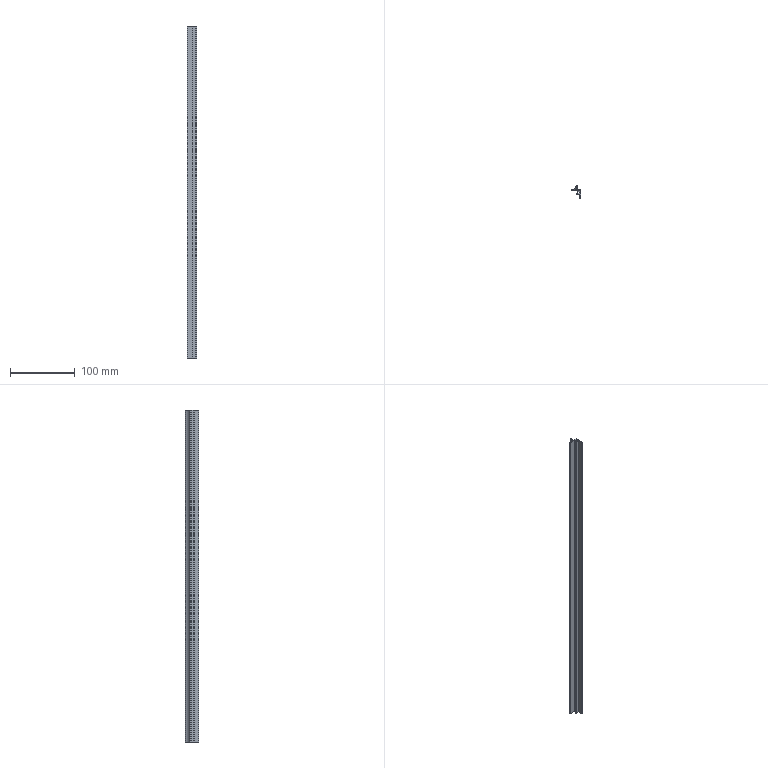Part | SolidWorks | features BaseBody 1, ICE 1, MoveFace 1 | 1 solid | 27 faces | box 14 x 20.3 x 513 mm | volume 26120 mm3 | plane 20 | cylinder 7 | commonest cylinder face diameters 0.387 x2 0.8 x2 0.4 x1 20 x1 22 x1
STEP:
#1=CARTESIAN_POINT('',(-5.304,-0.625,200.));
#2=VERTEX_POINT('',#1);
#3=CARTESIAN_POINT('',(-5.449,-0.8125,200.));
#4=VERTEX_POINT('',#3);
#5=CARTESIAN_POINT('',(-5.255,-0.8125,200.));
#6=DIRECTION('',(0.,0.,1.));
#7=DIRECTION('',(-1.,0.,0.));
#8=AXIS2_PLACEMENT_3D('',#5,#6,#7);
#9=CIRCLE('',#8,0.1937);
#10=EDGE_CURVE('',#2,#4,#9,.T.);
#11=ORIENTED_EDGE('',*,*,#10,.T.);
#12=CARTESIAN_POINT('',(-5.449,-0.8125,-313.));
#13=VERTEX_POINT('',#12);
#14=CARTESIAN_POINT('',(-5.449,-0.8125,230.));
#15=DIRECTION('',(0.,0.,-1.));
#16=VECTOR('',#15,1000.);
#17=LINE('',#14,#16);
#18=EDGE_CURVE('',#4,#13,#17,.T.);
#19=ORIENTED_EDGE('',*,*,#18,.T.);
#20=CARTESIAN_POINT('',(-5.304,-0.625,-313.));
#21=VERTEX_POINT('',#20);
#22=CARTESIAN_POINT('',(-5.255,-0.8125,-313.));
#23=DIRECTION('',(0.,0.,-1.));
#24=DIRECTION('',(1.,0.,0.));
#25=AXIS2_PLACEMENT_3D('',#22,#23,#24);
#26=CIRCLE('',#25,0.1937);
#27=EDGE_CURVE('',#13,#21,#26,.T.);
#28=ORIENTED_EDGE('',*,*,#27,.T.);
#29=CARTESIAN_POINT('',(-5.304,-0.625,230.));
#30=DIRECTION('',(0.,0.,-1.));
#31=VECTOR('',#30,1000.);
#32=LINE('',#29,#31);
#33=EDGE_CURVE('',#2,#21,#32,.T.);
#34=ORIENTED_EDGE('',*,*,#33,.F.);
#35=EDGE_LOOP('',(#11,#19,#28,#34));
#36=FACE_OUTER_BOUND('',#35,.T.);
#37=CARTESIAN_POINT('',(-5.255,-0.8125,230.));
#38=DIRECTION('',(0.,0.,-1.));
#39=DIRECTION('',(-1.,0.,0.));
#40=AXIS2_PLACEMENT_3D('',#37,#38,#39);
#41=CYLINDRICAL_SURFACE('',#40,0.1937);
#42=ADVANCED_FACE('',(#36),#41,.F.);
#43=CARTESIAN_POINT('',(5.,-1.,-313.));
#44=VERTEX_POINT('',#43);
#45=CARTESIAN_POINT('',(5.,-14.3,-313.));
#46=VERTEX_POINT('',#45);
#47=CARTESIAN_POINT('',(5.,29.623,-313.));
#48=DIRECTION('',(0.,-1.,0.));
#49=VECTOR('',#48,1000.);
#50=LINE('',#47,#49);
#51=EDGE_CURVE('',#44,#46,#50,.T.);
#52=ORIENTED_EDGE('',*,*,#51,.F.);
#53=CARTESIAN_POINT('',(5.,-1.,200.));
#54=VERTEX_POINT('',#53);
#55=CARTESIAN_POINT('',(5.,-1.,230.));
#56=DIRECTION('',(0.,0.,-1.));
#57=VECTOR('',#56,1000.);
#58=LINE('',#55,#57);
#59=EDGE_CURVE('',#54,#44,#58,.T.);
#60=ORIENTED_EDGE('',*,*,#59,.F.);
#61=CARTESIAN_POINT('',(5.,-14.3,200.));
#62=VERTEX_POINT('',#61);
#63=CARTESIAN_POINT('',(5.,-14.3,200.));
#64=DIRECTION('',(0.,1.,0.));
#65=VECTOR('',#64,1000.);
#66=LINE('',#63,#65);
#67=EDGE_CURVE('',#62,#54,#66,.T.);
#68=ORIENTED_EDGE('',*,*,#67,.F.);
#69=CARTESIAN_POINT('',(5.,-14.3,230.));
#70=DIRECTION('',(0.,0.,1.));
#71=VECTOR('',#70,1000.);
#72=LINE('',#69,#71);
#73=EDGE_CURVE('',#46,#62,#72,.T.);
#74=ORIENTED_EDGE('',*,*,#73,.F.);
#75=EDGE_LOOP('',(#52,#60,#68,#74));
#76=FACE_OUTER_BOUND('',#75,.T.);
#77=CARTESIAN_POINT('',(5.,-14.3,230.));
#78=DIRECTION('',(-1.,0.,0.));
#79=DIRECTION('',(0.,0.,1.));
#80=AXIS2_PLACEMENT_3D('',#77,#78,#79);
#81=PLANE('',#80);
#82=ADVANCED_FACE('',(#76),#81,.F.);
#83=CARTESIAN_POINT('',(-9.,-2.,-313.));
#84=VERTEX_POINT('',#83);
#85=CARTESIAN_POINT('',(-9.,-2.,200.));
#86=VERTEX_POINT('',#85);
#87=CARTESIAN_POINT('',(-9.,-2.,230.));
#88=DIRECTION('',(0.,0.,1.));
#89=VECTOR('',#88,1000.);
#90=LINE('',#87,#89);
#91=EDGE_CURVE('',#84,#86,#90,.T.);
#92=ORIENTED_EDGE('',*,*,#91,.F.);
#93=CARTESIAN_POINT('',(0.9,-2.,-313.));
#94=VERTEX_POINT('',#93);
#95=CARTESIAN_POINT('',(5.,-2.,-313.));
#96=DIRECTION('',(-1.,0.,0.));
#97=VECTOR('',#96,1000.);
#98=LINE('',#95,#97);
#99=EDGE_CURVE('',#94,#84,#98,.T.);
#100=ORIENTED_EDGE('',*,*,#99,.F.);
#101=CARTESIAN_POINT('',(0.9,-2.,200.));
#102=VERTEX_POINT('',#101);
#103=CARTESIAN_POINT('',(0.9,-2.,230.));
#104=DIRECTION('',(0.,0.,-1.));
#105=VECTOR('',#104,1000.);
#106=LINE('',#103,#105);
#107=EDGE_CURVE('',#102,#94,#106,.T.);
#108=ORIENTED_EDGE('',*,*,#107,.F.);
#109=CARTESIAN_POINT('',(5.,-2.,200.));
#110=DIRECTION('',(1.,0.,0.));
#111=VECTOR('',#110,1000.);
#112=LINE('',#109,#111);
#113=EDGE_CURVE('',#86,#102,#112,.T.);
#114=ORIENTED_EDGE('',*,*,#113,.F.);
#115=EDGE_LOOP('',(#92,#100,#108,#114));
#116=FACE_OUTER_BOUND('',#115,.T.);
#117=CARTESIAN_POINT('',(-9.,-2.,230.));
#118=DIRECTION('',(0.,1.,0.));
#119=DIRECTION('',(0.,0.,1.));
#120=AXIS2_PLACEMENT_3D('',#117,#118,#119);
#121=PLANE('',#120);
#122=ADVANCED_FACE('',(#116),#121,.F.);
#123=CARTESIAN_POINT('',(4.,-6.,200.));
#124=VERTEX_POINT('',#123);
#125=CARTESIAN_POINT('',(4.,-3.,200.));
#126=VERTEX_POINT('',#125);
#127=CARTESIAN_POINT('',(4.,29.623,200.));
#128=DIRECTION('',(0.,1.,0.));
#129=VECTOR('',#128,1000.);
#130=LINE('',#127,#129);
#131=EDGE_CURVE('',#124,#126,#130,.T.);
#132=ORIENTED_EDGE('',*,*,#131,.F.);
#133=CARTESIAN_POINT('',(1.,-6.,200.));
#134=VERTEX_POINT('',#133);
#135=CARTESIAN_POINT('',(5.,-6.,200.));
#136=DIRECTION('',(1.,0.,0.));
#137=VECTOR('',#136,1000.);
#138=LINE('',#135,#137);
#139=EDGE_CURVE('',#134,#124,#138,.T.);
#140=ORIENTED_EDGE('',*,*,#139,.F.);
#141=CARTESIAN_POINT('',(1.,-6.7,200.));
#142=VERTEX_POINT('',#141);
#143=CARTESIAN_POINT('',(1.,-6.,200.));
#144=DIRECTION('',(0.,-1.,0.));
#145=VECTOR('',#144,1000.);
#146=LINE('',#143,#145);
#147=EDGE_CURVE('',#134,#142,#146,.T.);
#148=ORIENTED_EDGE('',*,*,#147,.T.);
#149=CARTESIAN_POINT('',(-1.7,-6.7,200.));
#150=VERTEX_POINT('',#149);
#151=CARTESIAN_POINT('',(5.,-6.7,200.));
#152=DIRECTION('',(1.,0.,0.));
#153=VECTOR('',#152,1000.);
#154=LINE('',#151,#153);
#155=EDGE_CURVE('',#150,#142,#154,.T.);
#156=ORIENTED_EDGE('',*,*,#155,.F.);
#157=CARTESIAN_POINT('',(-1.7,-7.7,200.));
#158=VERTEX_POINT('',#157);
#159=CARTESIAN_POINT('',(-1.7,-6.7,200.));
#160=DIRECTION('',(0.,-1.,0.));
#161=VECTOR('',#160,1000.);
#162=LINE('',#159,#161);
#163=EDGE_CURVE('',#150,#158,#162,.T.);
#164=ORIENTED_EDGE('',*,*,#163,.T.);
#165=CARTESIAN_POINT('',(4.,-7.7,200.));
#166=VERTEX_POINT('',#165);
#167=CARTESIAN_POINT('',(5.,-7.7,200.));
#168=DIRECTION('',(-1.,0.,0.));
#169=VECTOR('',#168,1000.);
#170=LINE('',#167,#169);
#171=EDGE_CURVE('',#166,#158,#170,.T.);
#172=ORIENTED_EDGE('',*,*,#171,.F.);
#173=CARTESIAN_POINT('',(4.,-14.3,200.));
#174=VERTEX_POINT('',#173);
#175=CARTESIAN_POINT('',(4.,29.623,200.));
#176=DIRECTION('',(0.,1.,0.));
#177=VECTOR('',#176,1000.);
#178=LINE('',#175,#177);
#179=EDGE_CURVE('',#174,#166,#178,.T.);
#180=ORIENTED_EDGE('',*,*,#179,.F.);
#181=CARTESIAN_POINT('',(5.,-14.3,200.));
#182=DIRECTION('',(-1.,0.,0.));
#183=VECTOR('',#182,1000.);
#184=LINE('',#181,#183);
#185=EDGE_CURVE('',#62,#174,#184,.T.);
#186=ORIENTED_EDGE('',*,*,#185,.F.);
#187=ORIENTED_EDGE('',*,*,#67,.T.);
#188=CARTESIAN_POINT('',(-5.207,-1.,200.));
#189=VERTEX_POINT('',#188);
#190=CARTESIAN_POINT('',(5.,-1.,200.));
#191=DIRECTION('',(1.,0.,0.));
#192=VECTOR('',#191,1000.);
#193=LINE('',#190,#192);
#194=EDGE_CURVE('',#189,#54,#193,.T.);
#195=ORIENTED_EDGE('',*,*,#194,.F.);
#196=CARTESIAN_POINT('',(-5.255,-0.8125,200.));
#197=DIRECTION('',(0.,0.,1.));
#198=DIRECTION('',(-1.,0.,0.));
#199=AXIS2_PLACEMENT_3D('',#196,#197,#198);
#200=CIRCLE('',#199,0.1937);
#201=EDGE_CURVE('',#4,#189,#200,.T.);
#202=ORIENTED_EDGE('',*,*,#201,.F.);
#203=ORIENTED_EDGE('',*,*,#10,.F.);
#204=CARTESIAN_POINT('',(-1.368,3.063,200.));
#205=VERTEX_POINT('',#204);
#206=CARTESIAN_POINT('',(-10.628,9.,200.));
#207=DIRECTION('',(0.,0.,1.));
#208=DIRECTION('',(-1.,0.,0.));
#209=AXIS2_PLACEMENT_3D('',#206,#207,#208);
#210=CIRCLE('',#209,11.);
#211=EDGE_CURVE('',#2,#205,#210,.T.);
#212=ORIENTED_EDGE('',*,*,#211,.T.);
#213=CARTESIAN_POINT('',(-1.,2.955,200.));
#214=VERTEX_POINT('',#213);
#215=CARTESIAN_POINT('',(-1.2,2.955,200.));
#216=DIRECTION('',(0.,0.,1.));
#217=DIRECTION('',(-1.,0.,0.));
#218=AXIS2_PLACEMENT_3D('',#215,#216,#217);
#219=CIRCLE('',#218,0.2);
#220=EDGE_CURVE('',#214,#205,#219,.T.);
#221=ORIENTED_EDGE('',*,*,#220,.F.);
#222=CARTESIAN_POINT('',(-1.,1.5,200.));
#223=VERTEX_POINT('',#222);
#224=CARTESIAN_POINT('',(-1.,2.955,200.));
#225=DIRECTION('',(0.,1.,0.));
#226=VECTOR('',#225,1000.);
#227=LINE('',#224,#226);
#228=EDGE_CURVE('',#223,#214,#227,.T.);
#229=ORIENTED_EDGE('',*,*,#228,.F.);
#230=CARTESIAN_POINT('',(0.,1.5,200.));
#231=VERTEX_POINT('',#230);
#232=CARTESIAN_POINT('',(-1.,1.5,200.));
#233=DIRECTION('',(-1.,0.,0.));
#234=VECTOR('',#233,1000.);
#235=LINE('',#232,#234);
#236=EDGE_CURVE('',#231,#223,#235,.T.);
#237=ORIENTED_EDGE('',*,*,#236,.F.);
#238=CARTESIAN_POINT('',(0.,6.,200.));
#239=VERTEX_POINT('',#238);
#240=CARTESIAN_POINT('',(0.,1.5,200.));
#241=DIRECTION('',(0.,-1.,0.));
#242=VECTOR('',#241,1000.);
#243=LINE('',#240,#242);
#244=EDGE_CURVE('',#239,#231,#243,.T.);
#245=ORIENTED_EDGE('',*,*,#244,.F.);
#246=CARTESIAN_POINT('',(-0.8,6.,200.));
#247=VERTEX_POINT('',#246);
#248=CARTESIAN_POINT('',(0.,6.,200.));
#249=DIRECTION('',(1.,0.,0.));
#250=VECTOR('',#249,1000.);
#251=LINE('',#248,#250);
#252=EDGE_CURVE('',#247,#239,#251,.T.);
#253=ORIENTED_EDGE('',*,*,#252,.F.);
#254=CARTESIAN_POINT('',(-1.178,5.731,200.));
#255=VERTEX_POINT('',#254);
#256=CARTESIAN_POINT('',(-0.8,5.6,200.));
#257=DIRECTION('',(0.,0.,1.));
#258=DIRECTION('',(-1.,0.,0.));
#259=AXIS2_PLACEMENT_3D('',#256,#257,#258);
#260=CIRCLE('',#259,0.4);
#261=EDGE_CURVE('',#247,#255,#260,.T.);
#262=ORIENTED_EDGE('',*,*,#261,.T.);
#263=CARTESIAN_POINT('',(-8.678,-0.8077,200.));
#264=VERTEX_POINT('',#263);
#265=CARTESIAN_POINT('',(-10.628,9.,200.));
#266=DIRECTION('',(0.,0.,1.));
#267=DIRECTION('',(-1.,0.,0.));
#268=AXIS2_PLACEMENT_3D('',#265,#266,#267);
#269=CIRCLE('',#268,10.);
#270=EDGE_CURVE('',#264,#255,#269,.T.);
#271=ORIENTED_EDGE('',*,*,#270,.F.);
#272=CARTESIAN_POINT('',(-9.,-1.2,200.));
#273=VERTEX_POINT('',#272);
#274=CARTESIAN_POINT('',(-8.6,-1.2,200.));
#275=DIRECTION('',(0.,0.,1.));
#276=DIRECTION('',(-1.,0.,0.));
#277=AXIS2_PLACEMENT_3D('',#274,#275,#276);
#278=CIRCLE('',#277,0.4);
#279=EDGE_CURVE('',#264,#273,#278,.T.);
#280=ORIENTED_EDGE('',*,*,#279,.T.);
#281=CARTESIAN_POINT('',(-9.,8.,200.));
#282=DIRECTION('',(0.,-1.,0.));
#283=VECTOR('',#282,1000.);
#284=LINE('',#281,#283);
#285=EDGE_CURVE('',#273,#86,#284,.T.);
#286=ORIENTED_EDGE('',*,*,#285,.T.);
#287=ORIENTED_EDGE('',*,*,#113,.T.);
#288=CARTESIAN_POINT('',(0.9,-3.,200.));
#289=VERTEX_POINT('',#288);
#290=CARTESIAN_POINT('',(0.9,29.623,200.));
#291=DIRECTION('',(0.,1.,0.));
#292=VECTOR('',#291,1000.);
#293=LINE('',#290,#292);
#294=EDGE_CURVE('',#289,#102,#293,.T.);
#295=ORIENTED_EDGE('',*,*,#294,.F.);
#296=CARTESIAN_POINT('',(5.,-3.,200.));
#297=DIRECTION('',(-1.,0.,0.));
#298=VECTOR('',#297,1000.);
#299=LINE('',#296,#298);
#300=EDGE_CURVE('',#126,#289,#299,.T.);
#301=ORIENTED_EDGE('',*,*,#300,.F.);
#302=EDGE_LOOP('',(#132,#140,#148,#156,#164,#172,#180,#186,#187,#195,#202,#203,#212,#221,#229,#237,#245,#253,#262,#271,#280,#286,#287,#295,#301));
#303=FACE_OUTER_BOUND('',#302,.T.);
#304=CARTESIAN_POINT('',(5.,29.623,200.));
#305=DIRECTION('',(0.,0.,-1.));
#306=DIRECTION('',(-1.,0.,0.));
#307=AXIS2_PLACEMENT_3D('',#304,#305,#306);
#308=PLANE('',#307);
#309=ADVANCED_FACE('',(#303),#308,.F.);
#310=ORIENTED_EDGE('',*,*,#185,.T.);
#311=CARTESIAN_POINT('',(4.,-14.3,-313.));
#312=VERTEX_POINT('',#311);
#313=CARTESIAN_POINT('',(4.,-14.3,230.));
#314=DIRECTION('',(0.,0.,1.));
#315=VECTOR('',#314,1000.);
#316=LINE('',#313,#315);
#317=EDGE_CURVE('',#312,#174,#316,.T.);
#318=ORIENTED_EDGE('',*,*,#317,.F.);
#319=CARTESIAN_POINT('',(5.,-14.3,-313.));
#320=DIRECTION('',(-1.,0.,0.));
#321=VECTOR('',#320,1000.);
#322=LINE('',#319,#321);
#323=EDGE_CURVE('',#46,#312,#322,.T.);
#324=ORIENTED_EDGE('',*,*,#323,.F.);
#325=ORIENTED_EDGE('',*,*,#73,.T.);
#326=EDGE_LOOP('',(#310,#318,#324,#325));
#327=FACE_OUTER_BOUND('',#326,.T.);
#328=CARTESIAN_POINT('',(4.,-14.3,230.));
#329=DIRECTION('',(0.,1.,0.));
#330=DIRECTION('',(0.,0.,1.));
#331=AXIS2_PLACEMENT_3D('',#328,#329,#330);
#332=PLANE('',#331);
#333=ADVANCED_FACE('',(#327),#332,.F.);
#334=ORIENTED_EDGE('',*,*,#51,.T.);
#335=ORIENTED_EDGE('',*,*,#323,.T.);
#336=CARTESIAN_POINT('',(4.,-7.7,-313.));
#337=VERTEX_POINT('',#336);
#338=CARTESIAN_POINT('',(4.,-7.7,-313.));
#339=DIRECTION('',(0.,-1.,0.));
#340=VECTOR('',#339,1000.);
#341=LINE('',#338,#340);
#342=EDGE_CURVE('',#337,#312,#341,.T.);
#343=ORIENTED_EDGE('',*,*,#342,.F.);
#344=CARTESIAN_POINT('',(-1.7,-7.7,-313.));
#345=VERTEX_POINT('',#344);
#346=CARTESIAN_POINT('',(-1.7,-7.7,-313.));
#347=DIRECTION('',(1.,0.,0.));
#348=VECTOR('',#347,1000.);
#349=LINE('',#346,#348);
#350=EDGE_CURVE('',#345,#337,#349,.T.);
#351=ORIENTED_EDGE('',*,*,#350,.F.);
#352=CARTESIAN_POINT('',(-1.7,-6.7,-313.));
#353=VERTEX_POINT('',#352);
#354=CARTESIAN_POINT('',(-1.7,29.623,-313.));
#355=DIRECTION('',(0.,1.,0.));
#356=VECTOR('',#355,1000.);
#357=LINE('',#354,#356);
#358=EDGE_CURVE('',#345,#353,#357,.T.);
#359=ORIENTED_EDGE('',*,*,#358,.T.);
#360=CARTESIAN_POINT('',(1.,-6.7,-313.));
#361=VERTEX_POINT('',#360);
#362=CARTESIAN_POINT('',(1.,-6.7,-313.));
#363=DIRECTION('',(-1.,0.,0.));
#364=VECTOR('',#363,1000.);
#365=LINE('',#362,#364);
#366=EDGE_CURVE('',#361,#353,#365,.T.);
#367=ORIENTED_EDGE('',*,*,#366,.F.);
#368=CARTESIAN_POINT('',(1.,-6.,-313.));
#369=VERTEX_POINT('',#368);
#370=CARTESIAN_POINT('',(1.,29.623,-313.));
#371=DIRECTION('',(0.,1.,0.));
#372=VECTOR('',#371,1000.);
#373=LINE('',#370,#372);
#374=EDGE_CURVE('',#361,#369,#373,.T.);
#375=ORIENTED_EDGE('',*,*,#374,.T.);
#376=CARTESIAN_POINT('',(4.,-6.,-313.));
#377=VERTEX_POINT('',#376);
#378=CARTESIAN_POINT('',(4.,-6.,-313.));
#379=DIRECTION('',(-1.,0.,0.));
#380=VECTOR('',#379,1000.);
#381=LINE('',#378,#380);
#382=EDGE_CURVE('',#377,#369,#381,.T.);
#383=ORIENTED_EDGE('',*,*,#382,.F.);
#384=CARTESIAN_POINT('',(4.,-3.,-313.));
#385=VERTEX_POINT('',#384);
#386=CARTESIAN_POINT('',(4.,-3.,-313.));
#387=DIRECTION('',(0.,-1.,0.));
#388=VECTOR('',#387,1000.);
#389=LINE('',#386,#388);
#390=EDGE_CURVE('',#385,#377,#389,.T.);
#391=ORIENTED_EDGE('',*,*,#390,.F.);
#392=CARTESIAN_POINT('',(0.9,-3.,-313.));
#393=VERTEX_POINT('',#392);
#394=CARTESIAN_POINT('',(0.9,-3.,-313.));
#395=DIRECTION('',(1.,0.,0.));
#396=VECTOR('',#395,1000.);
#397=LINE('',#394,#396);
#398=EDGE_CURVE('',#393,#385,#397,.T.);
#399=ORIENTED_EDGE('',*,*,#398,.F.);
#400=CARTESIAN_POINT('',(0.9,-2.,-313.));
#401=DIRECTION('',(0.,-1.,0.));
#402=VECTOR('',#401,1000.);
#403=LINE('',#400,#402);
#404=EDGE_CURVE('',#94,#393,#403,.T.);
#405=ORIENTED_EDGE('',*,*,#404,.F.);
#406=ORIENTED_EDGE('',*,*,#99,.T.);
#407=CARTESIAN_POINT('',(-9.,-1.2,-313.));
#408=VERTEX_POINT('',#407);
#409=CARTESIAN_POINT('',(-9.,-1.2,-313.));
#410=DIRECTION('',(0.,-1.,0.));
#411=VECTOR('',#410,1000.);
#412=LINE('',#409,#411);
#413=EDGE_CURVE('',#408,#84,#412,.T.);
#414=ORIENTED_EDGE('',*,*,#413,.F.);
#415=CARTESIAN_POINT('',(-8.678,-0.8077,-313.));
#416=VERTEX_POINT('',#415);
#417=CARTESIAN_POINT('',(-8.6,-1.2,-313.));
#418=DIRECTION('',(0.,0.,-1.));
#419=DIRECTION('',(1.,0.,0.));
#420=AXIS2_PLACEMENT_3D('',#417,#418,#419);
#421=CIRCLE('',#420,0.4);
#422=EDGE_CURVE('',#408,#416,#421,.T.);
#423=ORIENTED_EDGE('',*,*,#422,.T.);
#424=CARTESIAN_POINT('',(-1.178,5.731,-313.));
#425=VERTEX_POINT('',#424);
#426=CARTESIAN_POINT('',(-10.628,9.,-313.));
#427=DIRECTION('',(0.,0.,-1.));
#428=DIRECTION('',(1.,0.,0.));
#429=AXIS2_PLACEMENT_3D('',#426,#427,#428);
#430=CIRCLE('',#429,10.);
#431=EDGE_CURVE('',#425,#416,#430,.T.);
#432=ORIENTED_EDGE('',*,*,#431,.F.);
#433=CARTESIAN_POINT('',(-0.8,6.,-313.));
#434=VERTEX_POINT('',#433);
#435=CARTESIAN_POINT('',(-0.8,5.6,-313.));
#436=DIRECTION('',(0.,0.,-1.));
#437=DIRECTION('',(1.,0.,0.));
#438=AXIS2_PLACEMENT_3D('',#435,#436,#437);
#439=CIRCLE('',#438,0.4);
#440=EDGE_CURVE('',#425,#434,#439,.T.);
#441=ORIENTED_EDGE('',*,*,#440,.T.);
#442=CARTESIAN_POINT('',(0.,6.,-313.));
#443=VERTEX_POINT('',#442);
#444=CARTESIAN_POINT('',(0.,6.,-313.));
#445=DIRECTION('',(-1.,0.,0.));
#446=VECTOR('',#445,1000.);
#447=LINE('',#444,#446);
#448=EDGE_CURVE('',#443,#434,#447,.T.);
#449=ORIENTED_EDGE('',*,*,#448,.F.);
#450=CARTESIAN_POINT('',(0.,1.5,-313.));
#451=VERTEX_POINT('',#450);
#452=CARTESIAN_POINT('',(0.,1.5,-313.));
#453=DIRECTION('',(0.,1.,0.));
#454=VECTOR('',#453,1000.);
#455=LINE('',#452,#454);
#456=EDGE_CURVE('',#451,#443,#455,.T.);
#457=ORIENTED_EDGE('',*,*,#456,.F.);
#458=CARTESIAN_POINT('',(-1.,1.5,-313.));
#459=VERTEX_POINT('',#458);
#460=CARTESIAN_POINT('',(-1.,1.5,-313.));
#461=DIRECTION('',(1.,0.,0.));
#462=VECTOR('',#461,1000.);
#463=LINE('',#460,#462);
#464=EDGE_CURVE('',#459,#451,#463,.T.);
#465=ORIENTED_EDGE('',*,*,#464,.F.);
#466=CARTESIAN_POINT('',(-1.,2.955,-313.));
#467=VERTEX_POINT('',#466);
#468=CARTESIAN_POINT('',(-1.,2.955,-313.));
#469=DIRECTION('',(0.,-1.,0.));
#470=VECTOR('',#469,1000.);
#471=LINE('',#468,#470);
#472=EDGE_CURVE('',#467,#459,#471,.T.);
#473=ORIENTED_EDGE('',*,*,#472,.F.);
#474=CARTESIAN_POINT('',(-1.368,3.063,-313.));
#475=VERTEX_POINT('',#474);
#476=CARTESIAN_POINT('',(-1.2,2.955,-313.));
#477=DIRECTION('',(0.,0.,-1.));
#478=DIRECTION('',(1.,0.,0.));
#479=AXIS2_PLACEMENT_3D('',#476,#477,#478);
#480=CIRCLE('',#479,0.2);
#481=EDGE_CURVE('',#475,#467,#480,.T.);
#482=ORIENTED_EDGE('',*,*,#481,.F.);
#483=CARTESIAN_POINT('',(-10.628,9.,-313.));
#484=DIRECTION('',(0.,0.,-1.));
#485=DIRECTION('',(1.,0.,0.));
#486=AXIS2_PLACEMENT_3D('',#483,#484,#485);
#487=CIRCLE('',#486,11.);
#488=EDGE_CURVE('',#475,#21,#487,.T.);
#489=ORIENTED_EDGE('',*,*,#488,.T.);
#490=ORIENTED_EDGE('',*,*,#27,.F.);
#491=CARTESIAN_POINT('',(-5.207,-1.,-313.));
#492=VERTEX_POINT('',#491);
#493=CARTESIAN_POINT('',(-5.255,-0.8125,-313.));
#494=DIRECTION('',(0.,0.,-1.));
#495=DIRECTION('',(1.,0.,0.));
#496=AXIS2_PLACEMENT_3D('',#493,#494,#495);
#497=CIRCLE('',#496,0.1937);
#498=EDGE_CURVE('',#492,#13,#497,.T.);
#499=ORIENTED_EDGE('',*,*,#498,.F.);
#500=CARTESIAN_POINT('',(5.,-1.,-313.));
#501=DIRECTION('',(-1.,0.,0.));
#502=VECTOR('',#501,1000.);
#503=LINE('',#500,#502);
#504=EDGE_CURVE('',#44,#492,#503,.T.);
#505=ORIENTED_EDGE('',*,*,#504,.F.);
#506=EDGE_LOOP('',(#334,#335,#343,#351,#359,#367,#375,#383,#391,#399,#405,#406,#414,#423,#432,#441,#449,#457,#465,#473,#482,#489,#490,#499,#505));
#507=FACE_OUTER_BOUND('',#506,.T.);
#508=CARTESIAN_POINT('',(5.,29.623,-313.));
#509=DIRECTION('',(0.,0.,1.));
#510=DIRECTION('',(1.,0.,0.));
#511=AXIS2_PLACEMENT_3D('',#508,#509,#510);
#512=PLANE('',#511);
#513=ADVANCED_FACE('',(#507),#512,.F.);
#514=ORIENTED_EDGE('',*,*,#59,.T.);
#515=ORIENTED_EDGE('',*,*,#504,.T.);
#516=CARTESIAN_POINT('',(-5.207,-1.,230.));
#517=DIRECTION('',(0.,0.,-1.));
#518=VECTOR('',#517,1000.);
#519=LINE('',#516,#518);
#520=EDGE_CURVE('',#189,#492,#519,.T.);
#521=ORIENTED_EDGE('',*,*,#520,.F.);
#522=ORIENTED_EDGE('',*,*,#194,.T.);
#523=EDGE_LOOP('',(#514,#515,#521,#522));
#524=FACE_OUTER_BOUND('',#523,.T.);
#525=CARTESIAN_POINT('',(5.,-1.,230.));
#526=DIRECTION('',(0.,-1.,0.));
#527=DIRECTION('',(0.,0.,-1.));
#528=AXIS2_PLACEMENT_3D('',#525,#526,#527);
#529=PLANE('',#528);
#530=ADVANCED_FACE('',(#524),#529,.F.);
#531=CARTESIAN_POINT('',(-9.,-1.2,230.));
#532=DIRECTION('',(0.,0.,1.));
#533=VECTOR('',#532,1000.);
#534=LINE('',#531,#533);
#535=EDGE_CURVE('',#408,#273,#534,.T.);
#536=ORIENTED_EDGE('',*,*,#535,.F.);
#537=ORIENTED_EDGE('',*,*,#413,.T.);
#538=ORIENTED_EDGE('',*,*,#91,.T.);
#539=ORIENTED_EDGE('',*,*,#285,.F.);
#540=EDGE_LOOP('',(#536,#537,#538,#539));
#541=FACE_OUTER_BOUND('',#540,.T.);
#542=CARTESIAN_POINT('',(-9.,-1.2,230.));
#543=DIRECTION('',(1.,0.,0.));
#544=DIRECTION('',(0.,0.,-1.));
#545=AXIS2_PLACEMENT_3D('',#542,#543,#544);
#546=PLANE('',#545);
#547=ADVANCED_FACE('',(#541),#546,.F.);
#548=ORIENTED_EDGE('',*,*,#294,.T.);
#549=ORIENTED_EDGE('',*,*,#107,.T.);
#550=ORIENTED_EDGE('',*,*,#404,.T.);
#551=CARTESIAN_POINT('',(0.9,-3.,230.));
#552=DIRECTION('',(0.,0.,-1.));
#553=VECTOR('',#552,1000.);
#554=LINE('',#551,#553);
#555=EDGE_CURVE('',#289,#393,#554,.T.);
#556=ORIENTED_EDGE('',*,*,#555,.F.);
#557=EDGE_LOOP('',(#548,#549,#550,#556));
#558=FACE_OUTER_BOUND('',#557,.T.);
#559=CARTESIAN_POINT('',(0.9,-2.,230.));
#560=DIRECTION('',(1.,0.,0.));
#561=DIRECTION('',(0.,0.,-1.));
#562=AXIS2_PLACEMENT_3D('',#559,#560,#561);
#563=PLANE('',#562);
#564=ADVANCED_FACE('',(#558),#563,.F.);
#565=ORIENTED_EDGE('',*,*,#300,.T.);
#566=ORIENTED_EDGE('',*,*,#555,.T.);
#567=ORIENTED_EDGE('',*,*,#398,.T.);
#568=CARTESIAN_POINT('',(4.,-3.,230.));
#569=DIRECTION('',(0.,0.,-1.));
#570=VECTOR('',#569,1000.);
#571=LINE('',#568,#570);
#572=EDGE_CURVE('',#126,#385,#571,.T.);
#573=ORIENTED_EDGE('',*,*,#572,.F.);
#574=EDGE_LOOP('',(#565,#566,#567,#573));
#575=FACE_OUTER_BOUND('',#574,.T.);
#576=CARTESIAN_POINT('',(0.9,-3.,230.));
#577=DIRECTION('',(0.,1.,0.));
#578=DIRECTION('',(0.,0.,1.));
#579=AXIS2_PLACEMENT_3D('',#576,#577,#578);
#580=PLANE('',#579);
#581=ADVANCED_FACE('',(#575),#580,.F.);
#582=ORIENTED_EDGE('',*,*,#131,.T.);
#583=ORIENTED_EDGE('',*,*,#572,.T.);
#584=ORIENTED_EDGE('',*,*,#390,.T.);
#585=CARTESIAN_POINT('',(4.,-6.,230.));
#586=DIRECTION('',(0.,0.,-1.));
#587=VECTOR('',#586,1000.);
#588=LINE('',#585,#587);
#589=EDGE_CURVE('',#124,#377,#588,.T.);
#590=ORIENTED_EDGE('',*,*,#589,.F.);
#591=EDGE_LOOP('',(#582,#583,#584,#590));
#592=FACE_OUTER_BOUND('',#591,.T.);
#593=CARTESIAN_POINT('',(4.,-3.,230.));
#594=DIRECTION('',(1.,0.,0.));
#595=DIRECTION('',(0.,0.,-1.));
#596=AXIS2_PLACEMENT_3D('',#593,#594,#595);
#597=PLANE('',#596);
#598=ADVANCED_FACE('',(#592),#597,.F.);
#599=ORIENTED_EDGE('',*,*,#139,.T.);
#600=ORIENTED_EDGE('',*,*,#589,.T.);
#601=ORIENTED_EDGE('',*,*,#382,.T.);
#602=CARTESIAN_POINT('',(1.,-6.,230.));
#603=DIRECTION('',(0.,0.,-1.));
#604=VECTOR('',#603,1000.);
#605=LINE('',#602,#604);
#606=EDGE_CURVE('',#134,#369,#605,.T.);
#607=ORIENTED_EDGE('',*,*,#606,.F.);
#608=EDGE_LOOP('',(#599,#600,#601,#607));
#609=FACE_OUTER_BOUND('',#608,.T.);
#610=CARTESIAN_POINT('',(4.,-6.,230.));
#611=DIRECTION('',(0.,-1.,0.));
#612=DIRECTION('',(0.,0.,-1.));
#613=AXIS2_PLACEMENT_3D('',#610,#611,#612);
#614=PLANE('',#613);
#615=ADVANCED_FACE('',(#609),#614,.F.);
#616=ORIENTED_EDGE('',*,*,#155,.T.);
#617=CARTESIAN_POINT('',(1.,-6.7,230.));
#618=DIRECTION('',(0.,0.,1.));
#619=VECTOR('',#618,1000.);
#620=LINE('',#617,#619);
#621=EDGE_CURVE('',#361,#142,#620,.T.);
#622=ORIENTED_EDGE('',*,*,#621,.F.);
#623=ORIENTED_EDGE('',*,*,#366,.T.);
#624=CARTESIAN_POINT('',(-1.7,-6.7,230.));
#625=DIRECTION('',(0.,0.,-1.));
#626=VECTOR('',#625,1000.);
#627=LINE('',#624,#626);
#628=EDGE_CURVE('',#150,#353,#627,.T.);
#629=ORIENTED_EDGE('',*,*,#628,.F.);
#630=EDGE_LOOP('',(#616,#622,#623,#629));
#631=FACE_OUTER_BOUND('',#630,.T.);
#632=CARTESIAN_POINT('',(1.,-6.7,230.));
#633=DIRECTION('',(0.,-1.,0.));
#634=DIRECTION('',(0.,0.,-1.));
#635=AXIS2_PLACEMENT_3D('',#632,#633,#634);
#636=PLANE('',#635);
#637=ADVANCED_FACE('',(#631),#636,.F.);
#638=ORIENTED_EDGE('',*,*,#171,.T.);
#639=CARTESIAN_POINT('',(-1.7,-7.7,230.));
#640=DIRECTION('',(0.,0.,1.));
#641=VECTOR('',#640,1000.);
#642=LINE('',#639,#641);
#643=EDGE_CURVE('',#345,#158,#642,.T.);
#644=ORIENTED_EDGE('',*,*,#643,.F.);
#645=ORIENTED_EDGE('',*,*,#350,.T.);
#646=CARTESIAN_POINT('',(4.,-7.7,230.));
#647=DIRECTION('',(0.,0.,-1.));
#648=VECTOR('',#647,1000.);
#649=LINE('',#646,#648);
#650=EDGE_CURVE('',#166,#337,#649,.T.);
#651=ORIENTED_EDGE('',*,*,#650,.F.);
#652=EDGE_LOOP('',(#638,#644,#645,#651));
#653=FACE_OUTER_BOUND('',#652,.T.);
#654=CARTESIAN_POINT('',(-1.7,-7.7,230.));
#655=DIRECTION('',(0.,1.,0.));
#656=DIRECTION('',(0.,0.,1.));
#657=AXIS2_PLACEMENT_3D('',#654,#655,#656);
#658=PLANE('',#657);
#659=ADVANCED_FACE('',(#653),#658,.F.);
#660=ORIENTED_EDGE('',*,*,#179,.T.);
#661=ORIENTED_EDGE('',*,*,#650,.T.);
#662=ORIENTED_EDGE('',*,*,#342,.T.);
#663=ORIENTED_EDGE('',*,*,#317,.T.);
#664=EDGE_LOOP('',(#660,#661,#662,#663));
#665=FACE_OUTER_BOUND('',#664,.T.);
#666=CARTESIAN_POINT('',(4.,-7.7,230.));
#667=DIRECTION('',(1.,0.,0.));
#668=DIRECTION('',(0.,0.,-1.));
#669=AXIS2_PLACEMENT_3D('',#666,#667,#668);
#670=PLANE('',#669);
#671=ADVANCED_FACE('',(#665),#670,.F.);
#672=ORIENTED_EDGE('',*,*,#18,.F.);
#673=ORIENTED_EDGE('',*,*,#201,.T.);
#674=ORIENTED_EDGE('',*,*,#520,.T.);
#675=ORIENTED_EDGE('',*,*,#498,.T.);
#676=EDGE_LOOP('',(#672,#673,#674,#675));
#677=FACE_OUTER_BOUND('',#676,.T.);
#678=CARTESIAN_POINT('',(-5.255,-0.8125,230.));
#679=DIRECTION('',(0.,0.,-1.));
#680=DIRECTION('',(-1.,0.,0.));
#681=AXIS2_PLACEMENT_3D('',#678,#679,#680);
#682=CYLINDRICAL_SURFACE('',#681,0.1937);
#683=ADVANCED_FACE('',(#677),#682,.F.);
#684=CARTESIAN_POINT('',(-1.,2.955,230.));
#685=DIRECTION('',(0.,0.,1.));
#686=VECTOR('',#685,1000.);
#687=LINE('',#684,#686);
#688=EDGE_CURVE('',#467,#214,#687,.T.);
#689=ORIENTED_EDGE('',*,*,#688,.F.);
#690=ORIENTED_EDGE('',*,*,#472,.T.);
#691=CARTESIAN_POINT('',(-1.,1.5,230.));
#692=DIRECTION('',(0.,0.,-1.));
#693=VECTOR('',#692,1000.);
#694=LINE('',#691,#693);
#695=EDGE_CURVE('',#223,#459,#694,.T.);
#696=ORIENTED_EDGE('',*,*,#695,.F.);
#697=ORIENTED_EDGE('',*,*,#228,.T.);
#698=EDGE_LOOP('',(#689,#690,#696,#697));
#699=FACE_OUTER_BOUND('',#698,.T.);
#700=CARTESIAN_POINT('',(-1.,2.955,230.));
#701=DIRECTION('',(1.,0.,0.));
#702=DIRECTION('',(0.,0.,-1.));
#703=AXIS2_PLACEMENT_3D('',#700,#701,#702);
#704=PLANE('',#703);
#705=ADVANCED_FACE('',(#699),#704,.F.);
#706=ORIENTED_EDGE('',*,*,#488,.F.);
#707=CARTESIAN_POINT('',(-1.368,3.063,230.));
#708=DIRECTION('',(0.,0.,1.));
#709=VECTOR('',#708,1000.);
#710=LINE('',#707,#709);
#711=EDGE_CURVE('',#475,#205,#710,.T.);
#712=ORIENTED_EDGE('',*,*,#711,.T.);
#713=ORIENTED_EDGE('',*,*,#211,.F.);
#714=ORIENTED_EDGE('',*,*,#33,.T.);
#715=EDGE_LOOP('',(#706,#712,#713,#714));
#716=FACE_OUTER_BOUND('',#715,.T.);
#717=CARTESIAN_POINT('',(-10.628,9.,230.));
#718=DIRECTION('',(0.,0.,-1.));
#719=DIRECTION('',(-1.,0.,0.));
#720=AXIS2_PLACEMENT_3D('',#717,#718,#719);
#721=CYLINDRICAL_SURFACE('',#720,11.);
#722=ADVANCED_FACE('',(#716),#721,.T.);
#723=CARTESIAN_POINT('',(-1.178,5.731,230.));
#724=DIRECTION('',(0.,0.,1.));
#725=VECTOR('',#724,1000.);
#726=LINE('',#723,#725);
#727=EDGE_CURVE('',#425,#255,#726,.T.);
#728=ORIENTED_EDGE('',*,*,#727,.F.);
#729=ORIENTED_EDGE('',*,*,#431,.T.);
#730=CARTESIAN_POINT('',(-8.678,-0.8077,230.));
#731=DIRECTION('',(0.,0.,-1.));
#732=VECTOR('',#731,1000.);
#733=LINE('',#730,#732);
#734=EDGE_CURVE('',#264,#416,#733,.T.);
#735=ORIENTED_EDGE('',*,*,#734,.F.);
#736=ORIENTED_EDGE('',*,*,#270,.T.);
#737=EDGE_LOOP('',(#728,#729,#735,#736));
#738=FACE_OUTER_BOUND('',#737,.T.);
#739=CARTESIAN_POINT('',(-10.628,9.,230.));
#740=DIRECTION('',(0.,0.,-1.));
#741=DIRECTION('',(-1.,0.,0.));
#742=AXIS2_PLACEMENT_3D('',#739,#740,#741);
#743=CYLINDRICAL_SURFACE('',#742,10.);
#744=ADVANCED_FACE('',(#738),#743,.F.);
#745=CARTESIAN_POINT('',(0.,1.5,230.));
#746=DIRECTION('',(0.,0.,1.));
#747=VECTOR('',#746,1000.);
#748=LINE('',#745,#747);
#749=EDGE_CURVE('',#451,#231,#748,.T.);
#750=ORIENTED_EDGE('',*,*,#749,.F.);
#751=ORIENTED_EDGE('',*,*,#456,.T.);
#752=CARTESIAN_POINT('',(0.,6.,230.));
#753=DIRECTION('',(0.,0.,-1.));
#754=VECTOR('',#753,1000.);
#755=LINE('',#752,#754);
#756=EDGE_CURVE('',#239,#443,#755,.T.);
#757=ORIENTED_EDGE('',*,*,#756,.F.);
#758=ORIENTED_EDGE('',*,*,#244,.T.);
#759=EDGE_LOOP('',(#750,#751,#757,#758));
#760=FACE_OUTER_BOUND('',#759,.T.);
#761=CARTESIAN_POINT('',(0.,1.5,230.));
#762=DIRECTION('',(-1.,0.,0.));
#763=DIRECTION('',(0.,0.,1.));
#764=AXIS2_PLACEMENT_3D('',#761,#762,#763);
#765=PLANE('',#764);
#766=ADVANCED_FACE('',(#760),#765,.F.);
#767=ORIENTED_EDGE('',*,*,#422,.F.);
#768=ORIENTED_EDGE('',*,*,#535,.T.);
#769=ORIENTED_EDGE('',*,*,#279,.F.);
#770=ORIENTED_EDGE('',*,*,#734,.T.);
#771=EDGE_LOOP('',(#767,#768,#769,#770));
#772=FACE_OUTER_BOUND('',#771,.T.);
#773=CARTESIAN_POINT('',(-8.6,-1.2,230.));
#774=DIRECTION('',(0.,0.,-1.));
#775=DIRECTION('',(-1.,0.,0.));
#776=AXIS2_PLACEMENT_3D('',#773,#774,#775);
#777=CYLINDRICAL_SURFACE('',#776,0.4);
#778=ADVANCED_FACE('',(#772),#777,.T.);
#779=ORIENTED_EDGE('',*,*,#147,.F.);
#780=ORIENTED_EDGE('',*,*,#606,.T.);
#781=ORIENTED_EDGE('',*,*,#374,.F.);
#782=ORIENTED_EDGE('',*,*,#621,.T.);
#783=EDGE_LOOP('',(#779,#780,#781,#782));
#784=FACE_OUTER_BOUND('',#783,.T.);
#785=CARTESIAN_POINT('',(1.,-6.,230.));
#786=DIRECTION('',(1.,0.,0.));
#787=DIRECTION('',(0.,0.,-1.));
#788=AXIS2_PLACEMENT_3D('',#785,#786,#787);
#789=PLANE('',#788);
#790=ADVANCED_FACE('',(#784),#789,.F.);
#791=ORIENTED_EDGE('',*,*,#163,.F.);
#792=ORIENTED_EDGE('',*,*,#628,.T.);
#793=ORIENTED_EDGE('',*,*,#358,.F.);
#794=ORIENTED_EDGE('',*,*,#643,.T.);
#795=EDGE_LOOP('',(#791,#792,#793,#794));
#796=FACE_OUTER_BOUND('',#795,.T.);
#797=CARTESIAN_POINT('',(-1.7,-6.7,230.));
#798=DIRECTION('',(1.,0.,0.));
#799=DIRECTION('',(0.,0.,-1.));
#800=AXIS2_PLACEMENT_3D('',#797,#798,#799);
#801=PLANE('',#800);
#802=ADVANCED_FACE('',(#796),#801,.F.);
#803=ORIENTED_EDGE('',*,*,#711,.F.);
#804=ORIENTED_EDGE('',*,*,#481,.T.);
#805=ORIENTED_EDGE('',*,*,#688,.T.);
#806=ORIENTED_EDGE('',*,*,#220,.T.);
#807=EDGE_LOOP('',(#803,#804,#805,#806));
#808=FACE_OUTER_BOUND('',#807,.T.);
#809=CARTESIAN_POINT('',(-1.2,2.955,230.));
#810=DIRECTION('',(0.,0.,-1.));
#811=DIRECTION('',(-1.,0.,0.));
#812=AXIS2_PLACEMENT_3D('',#809,#810,#811);
#813=CYLINDRICAL_SURFACE('',#812,0.2);
#814=ADVANCED_FACE('',(#808),#813,.F.);
#815=ORIENTED_EDGE('',*,*,#695,.T.);
#816=ORIENTED_EDGE('',*,*,#464,.T.);
#817=ORIENTED_EDGE('',*,*,#749,.T.);
#818=ORIENTED_EDGE('',*,*,#236,.T.);
#819=EDGE_LOOP('',(#815,#816,#817,#818));
#820=FACE_OUTER_BOUND('',#819,.T.);
#821=CARTESIAN_POINT('',(-1.,1.5,230.));
#822=DIRECTION('',(0.,1.,0.));
#823=DIRECTION('',(0.,0.,1.));
#824=AXIS2_PLACEMENT_3D('',#821,#822,#823);
#825=PLANE('',#824);
#826=ADVANCED_FACE('',(#820),#825,.F.);
#827=ORIENTED_EDGE('',*,*,#440,.F.);
#828=ORIENTED_EDGE('',*,*,#727,.T.);
#829=ORIENTED_EDGE('',*,*,#261,.F.);
#830=CARTESIAN_POINT('',(-0.8,6.,230.));
#831=DIRECTION('',(0.,0.,-1.));
#832=VECTOR('',#831,1000.);
#833=LINE('',#830,#832);
#834=EDGE_CURVE('',#247,#434,#833,.T.);
#835=ORIENTED_EDGE('',*,*,#834,.T.);
#836=EDGE_LOOP('',(#827,#828,#829,#835));
#837=FACE_OUTER_BOUND('',#836,.T.);
#838=CARTESIAN_POINT('',(-0.8,5.6,230.));
#839=DIRECTION('',(0.,0.,-1.));
#840=DIRECTION('',(-1.,0.,0.));
#841=AXIS2_PLACEMENT_3D('',#838,#839,#840);
#842=CYLINDRICAL_SURFACE('',#841,0.4);
#843=ADVANCED_FACE('',(#837),#842,.T.);
#844=ORIENTED_EDGE('',*,*,#756,.T.);
#845=ORIENTED_EDGE('',*,*,#448,.T.);
#846=ORIENTED_EDGE('',*,*,#834,.F.);
#847=ORIENTED_EDGE('',*,*,#252,.T.);
#848=EDGE_LOOP('',(#844,#845,#846,#847));
#849=FACE_OUTER_BOUND('',#848,.T.);
#850=CARTESIAN_POINT('',(0.,6.,230.));
#851=DIRECTION('',(0.,-1.,0.));
#852=DIRECTION('',(0.,0.,-1.));
#853=AXIS2_PLACEMENT_3D('',#850,#851,#852);
#854=PLANE('',#853);
#855=ADVANCED_FACE('',(#849),#854,.F.);
#856=CLOSED_SHELL('',(#42,#82,#122,#309,#333,#513,#530,#547,#564,#581,#598,#615,#637,#659,#671,#683,#705,#722,#744,#766,#778,#790,#802,#814,#826,#843,#855));
#857=MANIFOLD_SOLID_BREP('',#856);
#858=CARTESIAN_POINT('',(0.,0.,0.));
#859=DIRECTION('',(0.,0.,1.));
#860=DIRECTION('',(1.,0.,0.));
#861=AXIS2_PLACEMENT_3D('',#858,#859,#860);
#862=(LENGTH_UNIT()NAMED_UNIT(*)SI_UNIT(.MILLI.,.METRE.));
#863=UNCERTAINTY_MEASURE_WITH_UNIT(LENGTH_MEASURE(0.00001),#862,'','');
#864=(NAMED_UNIT(*)PLANE_ANGLE_UNIT()SI_UNIT($,.RADIAN.));
#865=(NAMED_UNIT(*)SI_UNIT($,.STERADIAN.)SOLID_ANGLE_UNIT());
#866=(GEOMETRIC_REPRESENTATION_CONTEXT(3)GLOBAL_UNCERTAINTY_ASSIGNED_CONTEXT((#863))GLOBAL_UNIT_ASSIGNED_CONTEXT((#862,#864,#865))REPRESENTATION_CONTEXT('',''));
#867=ADVANCED_BREP_SHAPE_REPRESENTATION('',(#857,#861),#866);